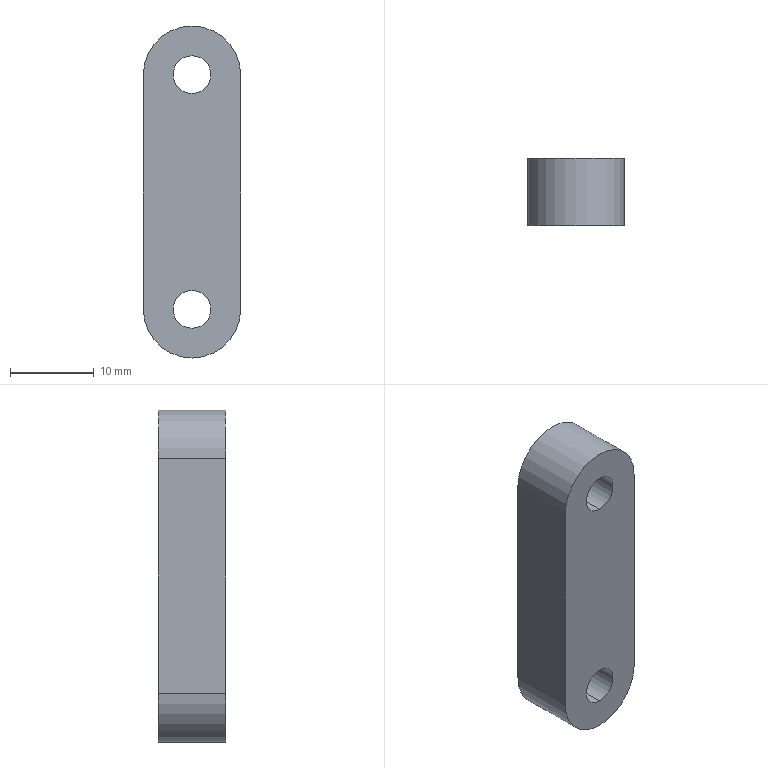Part | SolidWorks | features BaseBody 1 | 1 solid | 17 faces | box 11.6 x 8 x 39.6 mm | volume 2873 mm3 | cylinder 11 | plane 6 | commonest cylinder face diameters 4.5 x4 8 x4 11.6 x3
STEP:
#1=CARTESIAN_POINT('',(-5.8,8.,0.));
#2=VERTEX_POINT('',#1);
#3=CARTESIAN_POINT('',(0.,8.,-5.8));
#4=VERTEX_POINT('',#3);
#5=CARTESIAN_POINT('',(0.,8.,0.));
#6=DIRECTION('',(0.,-1.,0.));
#7=DIRECTION('',(0.,0.,-1.));
#8=AXIS2_PLACEMENT_3D('',#5,#6,#7);
#9=CIRCLE('',#8,5.8);
#10=EDGE_CURVE('',#2,#4,#9,.T.);
#11=ORIENTED_EDGE('',*,*,#10,.T.);
#12=CARTESIAN_POINT('',(0.,0.,-5.8));
#13=VERTEX_POINT('',#12);
#14=CARTESIAN_POINT('',(0.,8.,-5.8));
#15=DIRECTION('',(0.,-1.,0.));
#16=VECTOR('',#15,1000.);
#17=LINE('',#14,#16);
#18=EDGE_CURVE('',#4,#13,#17,.T.);
#19=ORIENTED_EDGE('',*,*,#18,.T.);
#20=CARTESIAN_POINT('',(-5.8,0.,0.));
#21=VERTEX_POINT('',#20);
#22=CARTESIAN_POINT('',(0.,0.,0.));
#23=DIRECTION('',(0.,1.,0.));
#24=DIRECTION('',(0.,0.,-1.));
#25=AXIS2_PLACEMENT_3D('',#22,#23,#24);
#26=CIRCLE('',#25,5.8);
#27=EDGE_CURVE('',#13,#21,#26,.T.);
#28=ORIENTED_EDGE('',*,*,#27,.T.);
#29=CARTESIAN_POINT('',(-5.8,8.,0.));
#30=DIRECTION('',(0.,1.,0.));
#31=VECTOR('',#30,1000.);
#32=LINE('',#29,#31);
#33=EDGE_CURVE('',#21,#2,#32,.T.);
#34=ORIENTED_EDGE('',*,*,#33,.T.);
#35=EDGE_LOOP('',(#11,#19,#28,#34));
#36=FACE_OUTER_BOUND('',#35,.T.);
#37=CARTESIAN_POINT('',(0.,8.,0.));
#38=DIRECTION('',(0.,-1.,0.));
#39=DIRECTION('',(0.,0.,-1.));
#40=AXIS2_PLACEMENT_3D('',#37,#38,#39);
#41=CYLINDRICAL_SURFACE('',#40,5.8);
#42=ADVANCED_FACE('',(#36),#41,.T.);
#43=CARTESIAN_POINT('',(0.,0.,30.25));
#44=VERTEX_POINT('',#43);
#45=CARTESIAN_POINT('',(0.,0.,25.75));
#46=VERTEX_POINT('',#45);
#47=CARTESIAN_POINT('',(0.,0.,28.));
#48=DIRECTION('',(0.,-1.,0.));
#49=DIRECTION('',(0.,0.,1.));
#50=AXIS2_PLACEMENT_3D('',#47,#48,#49);
#51=CIRCLE('',#50,2.25);
#52=EDGE_CURVE('',#44,#46,#51,.T.);
#53=ORIENTED_EDGE('',*,*,#52,.T.);
#54=CARTESIAN_POINT('',(0.,3.4,25.75));
#55=VERTEX_POINT('',#54);
#56=CARTESIAN_POINT('',(0.,8.,25.75));
#57=DIRECTION('',(0.,1.,0.));
#58=VECTOR('',#57,1000.);
#59=LINE('',#56,#58);
#60=EDGE_CURVE('',#46,#55,#59,.T.);
#61=ORIENTED_EDGE('',*,*,#60,.T.);
#62=CARTESIAN_POINT('',(0.,3.4,30.25));
#63=VERTEX_POINT('',#62);
#64=CARTESIAN_POINT('',(0.,3.4,28.));
#65=DIRECTION('',(0.,-1.,0.));
#66=DIRECTION('',(0.,0.,1.));
#67=AXIS2_PLACEMENT_3D('',#64,#65,#66);
#68=CIRCLE('',#67,2.25);
#69=EDGE_CURVE('',#63,#55,#68,.T.);
#70=ORIENTED_EDGE('',*,*,#69,.F.);
#71=CARTESIAN_POINT('',(0.,8.,30.25));
#72=DIRECTION('',(0.,1.,0.));
#73=VECTOR('',#72,1000.);
#74=LINE('',#71,#73);
#75=EDGE_CURVE('',#44,#63,#74,.T.);
#76=ORIENTED_EDGE('',*,*,#75,.F.);
#77=EDGE_LOOP('',(#53,#61,#70,#76));
#78=FACE_OUTER_BOUND('',#77,.T.);
#79=CARTESIAN_POINT('',(0.,8.,28.));
#80=DIRECTION('',(0.,1.,0.));
#81=DIRECTION('',(0.,0.,1.));
#82=AXIS2_PLACEMENT_3D('',#79,#80,#81);
#83=CYLINDRICAL_SURFACE('',#82,2.25);
#84=ADVANCED_FACE('',(#78),#83,.F.);
#85=CARTESIAN_POINT('',(0.,0.,2.25));
#86=VERTEX_POINT('',#85);
#87=CARTESIAN_POINT('',(0.,0.,-2.25));
#88=VERTEX_POINT('',#87);
#89=CARTESIAN_POINT('',(0.,0.,0.));
#90=DIRECTION('',(0.,-1.,0.));
#91=DIRECTION('',(0.,0.,1.));
#92=AXIS2_PLACEMENT_3D('',#89,#90,#91);
#93=CIRCLE('',#92,2.25);
#94=EDGE_CURVE('',#86,#88,#93,.T.);
#95=ORIENTED_EDGE('',*,*,#94,.T.);
#96=CARTESIAN_POINT('',(0.,3.4,-2.25));
#97=VERTEX_POINT('',#96);
#98=CARTESIAN_POINT('',(0.,8.,-2.25));
#99=DIRECTION('',(0.,1.,0.));
#100=VECTOR('',#99,1000.);
#101=LINE('',#98,#100);
#102=EDGE_CURVE('',#88,#97,#101,.T.);
#103=ORIENTED_EDGE('',*,*,#102,.T.);
#104=CARTESIAN_POINT('',(0.,3.4,2.25));
#105=VERTEX_POINT('',#104);
#106=CARTESIAN_POINT('',(0.,3.4,0.));
#107=DIRECTION('',(0.,-1.,0.));
#108=DIRECTION('',(0.,0.,1.));
#109=AXIS2_PLACEMENT_3D('',#106,#107,#108);
#110=CIRCLE('',#109,2.25);
#111=EDGE_CURVE('',#105,#97,#110,.T.);
#112=ORIENTED_EDGE('',*,*,#111,.F.);
#113=CARTESIAN_POINT('',(0.,8.,2.25));
#114=DIRECTION('',(0.,1.,0.));
#115=VECTOR('',#114,1000.);
#116=LINE('',#113,#115);
#117=EDGE_CURVE('',#86,#105,#116,.T.);
#118=ORIENTED_EDGE('',*,*,#117,.F.);
#119=EDGE_LOOP('',(#95,#103,#112,#118));
#120=FACE_OUTER_BOUND('',#119,.T.);
#121=CARTESIAN_POINT('',(0.,8.,0.));
#122=DIRECTION('',(0.,1.,0.));
#123=DIRECTION('',(0.,0.,1.));
#124=AXIS2_PLACEMENT_3D('',#121,#122,#123);
#125=CYLINDRICAL_SURFACE('',#124,2.25);
#126=ADVANCED_FACE('',(#120),#125,.F.);
#127=CARTESIAN_POINT('',(0.,3.4,32.));
#128=VERTEX_POINT('',#127);
#129=CARTESIAN_POINT('',(0.,3.4,24.));
#130=VERTEX_POINT('',#129);
#131=CARTESIAN_POINT('',(0.,3.4,28.));
#132=DIRECTION('',(0.,-1.,0.));
#133=DIRECTION('',(0.,0.,1.));
#134=AXIS2_PLACEMENT_3D('',#131,#132,#133);
#135=CIRCLE('',#134,4.);
#136=EDGE_CURVE('',#128,#130,#135,.T.);
#137=ORIENTED_EDGE('',*,*,#136,.T.);
#138=CARTESIAN_POINT('',(0.,8.,24.));
#139=VERTEX_POINT('',#138);
#140=CARTESIAN_POINT('',(0.,8.,24.));
#141=DIRECTION('',(0.,1.,0.));
#142=VECTOR('',#141,1000.);
#143=LINE('',#140,#142);
#144=EDGE_CURVE('',#130,#139,#143,.T.);
#145=ORIENTED_EDGE('',*,*,#144,.T.);
#146=CARTESIAN_POINT('',(0.,8.,32.));
#147=VERTEX_POINT('',#146);
#148=CARTESIAN_POINT('',(0.,8.,28.));
#149=DIRECTION('',(0.,-1.,0.));
#150=DIRECTION('',(0.,0.,1.));
#151=AXIS2_PLACEMENT_3D('',#148,#149,#150);
#152=CIRCLE('',#151,4.);
#153=EDGE_CURVE('',#147,#139,#152,.T.);
#154=ORIENTED_EDGE('',*,*,#153,.F.);
#155=CARTESIAN_POINT('',(0.,8.,32.));
#156=DIRECTION('',(0.,1.,0.));
#157=VECTOR('',#156,1000.);
#158=LINE('',#155,#157);
#159=EDGE_CURVE('',#128,#147,#158,.T.);
#160=ORIENTED_EDGE('',*,*,#159,.F.);
#161=EDGE_LOOP('',(#137,#145,#154,#160));
#162=FACE_OUTER_BOUND('',#161,.T.);
#163=CARTESIAN_POINT('',(0.,8.,28.));
#164=DIRECTION('',(0.,1.,0.));
#165=DIRECTION('',(0.,0.,1.));
#166=AXIS2_PLACEMENT_3D('',#163,#164,#165);
#167=CYLINDRICAL_SURFACE('',#166,4.);
#168=ADVANCED_FACE('',(#162),#167,.F.);
#169=CARTESIAN_POINT('',(0.,3.4,4.));
#170=VERTEX_POINT('',#169);
#171=CARTESIAN_POINT('',(0.,3.4,-4.));
#172=VERTEX_POINT('',#171);
#173=CARTESIAN_POINT('',(0.,3.4,0.));
#174=DIRECTION('',(0.,-1.,0.));
#175=DIRECTION('',(0.,0.,1.));
#176=AXIS2_PLACEMENT_3D('',#173,#174,#175);
#177=CIRCLE('',#176,4.);
#178=EDGE_CURVE('',#170,#172,#177,.T.);
#179=ORIENTED_EDGE('',*,*,#178,.T.);
#180=CARTESIAN_POINT('',(0.,8.,-4.));
#181=VERTEX_POINT('',#180);
#182=CARTESIAN_POINT('',(0.,8.,-4.));
#183=DIRECTION('',(0.,1.,0.));
#184=VECTOR('',#183,1000.);
#185=LINE('',#182,#184);
#186=EDGE_CURVE('',#172,#181,#185,.T.);
#187=ORIENTED_EDGE('',*,*,#186,.T.);
#188=CARTESIAN_POINT('',(0.,8.,4.));
#189=VERTEX_POINT('',#188);
#190=CARTESIAN_POINT('',(0.,8.,0.));
#191=DIRECTION('',(0.,-1.,0.));
#192=DIRECTION('',(0.,0.,1.));
#193=AXIS2_PLACEMENT_3D('',#190,#191,#192);
#194=CIRCLE('',#193,4.);
#195=EDGE_CURVE('',#189,#181,#194,.T.);
#196=ORIENTED_EDGE('',*,*,#195,.F.);
#197=CARTESIAN_POINT('',(0.,8.,4.));
#198=DIRECTION('',(0.,1.,0.));
#199=VECTOR('',#198,1000.);
#200=LINE('',#197,#199);
#201=EDGE_CURVE('',#170,#189,#200,.T.);
#202=ORIENTED_EDGE('',*,*,#201,.F.);
#203=EDGE_LOOP('',(#179,#187,#196,#202));
#204=FACE_OUTER_BOUND('',#203,.T.);
#205=CARTESIAN_POINT('',(0.,8.,0.));
#206=DIRECTION('',(0.,1.,0.));
#207=DIRECTION('',(0.,0.,1.));
#208=AXIS2_PLACEMENT_3D('',#205,#206,#207);
#209=CYLINDRICAL_SURFACE('',#208,4.);
#210=ADVANCED_FACE('',(#204),#209,.F.);
#211=CARTESIAN_POINT('',(5.8,0.,28.));
#212=VERTEX_POINT('',#211);
#213=CARTESIAN_POINT('',(5.8,0.,0.));
#214=VERTEX_POINT('',#213);
#215=CARTESIAN_POINT('',(5.8,0.,0.));
#216=DIRECTION('',(0.,0.,-1.));
#217=VECTOR('',#216,1000.);
#218=LINE('',#215,#217);
#219=EDGE_CURVE('',#212,#214,#218,.T.);
#220=ORIENTED_EDGE('',*,*,#219,.F.);
#221=CARTESIAN_POINT('',(-5.8,0.,28.));
#222=VERTEX_POINT('',#221);
#223=CARTESIAN_POINT('',(0.,0.,28.));
#224=DIRECTION('',(0.,1.,0.));
#225=DIRECTION('',(0.,0.,-1.));
#226=AXIS2_PLACEMENT_3D('',#223,#224,#225);
#227=CIRCLE('',#226,5.8);
#228=EDGE_CURVE('',#222,#212,#227,.T.);
#229=ORIENTED_EDGE('',*,*,#228,.F.);
#230=CARTESIAN_POINT('',(-5.8,0.,0.));
#231=DIRECTION('',(0.,0.,1.));
#232=VECTOR('',#231,1000.);
#233=LINE('',#230,#232);
#234=EDGE_CURVE('',#21,#222,#233,.T.);
#235=ORIENTED_EDGE('',*,*,#234,.F.);
#236=ORIENTED_EDGE('',*,*,#27,.F.);
#237=CARTESIAN_POINT('',(0.,0.,0.));
#238=DIRECTION('',(0.,1.,0.));
#239=DIRECTION('',(0.,0.,-1.));
#240=AXIS2_PLACEMENT_3D('',#237,#238,#239);
#241=CIRCLE('',#240,5.8);
#242=EDGE_CURVE('',#214,#13,#241,.T.);
#243=ORIENTED_EDGE('',*,*,#242,.F.);
#244=EDGE_LOOP('',(#220,#229,#235,#236,#243));
#245=FACE_OUTER_BOUND('',#244,.T.);
#246=ORIENTED_EDGE('',*,*,#52,.F.);
#247=CARTESIAN_POINT('',(0.,0.,28.));
#248=DIRECTION('',(0.,-1.,0.));
#249=DIRECTION('',(0.,0.,1.));
#250=AXIS2_PLACEMENT_3D('',#247,#248,#249);
#251=CIRCLE('',#250,2.25);
#252=EDGE_CURVE('',#46,#44,#251,.T.);
#253=ORIENTED_EDGE('',*,*,#252,.F.);
#254=EDGE_LOOP('',(#246,#253));
#255=FACE_BOUND('',#254,.T.);
#256=ORIENTED_EDGE('',*,*,#94,.F.);
#257=CARTESIAN_POINT('',(0.,0.,0.));
#258=DIRECTION('',(0.,-1.,0.));
#259=DIRECTION('',(0.,0.,1.));
#260=AXIS2_PLACEMENT_3D('',#257,#258,#259);
#261=CIRCLE('',#260,2.25);
#262=EDGE_CURVE('',#88,#86,#261,.T.);
#263=ORIENTED_EDGE('',*,*,#262,.F.);
#264=EDGE_LOOP('',(#256,#263));
#265=FACE_BOUND('',#264,.T.);
#266=CARTESIAN_POINT('',(0.,0.,0.));
#267=DIRECTION('',(0.,1.,0.));
#268=DIRECTION('',(0.,0.,1.));
#269=AXIS2_PLACEMENT_3D('',#266,#267,#268);
#270=PLANE('',#269);
#271=ADVANCED_FACE('',(#245,#255,#265),#270,.F.);
#272=ORIENTED_EDGE('',*,*,#18,.F.);
#273=CARTESIAN_POINT('',(5.8,8.,0.));
#274=VERTEX_POINT('',#273);
#275=CARTESIAN_POINT('',(0.,8.,0.));
#276=DIRECTION('',(0.,-1.,0.));
#277=DIRECTION('',(0.,0.,-1.));
#278=AXIS2_PLACEMENT_3D('',#275,#276,#277);
#279=CIRCLE('',#278,5.8);
#280=EDGE_CURVE('',#4,#274,#279,.T.);
#281=ORIENTED_EDGE('',*,*,#280,.T.);
#282=CARTESIAN_POINT('',(5.8,8.,0.));
#283=DIRECTION('',(0.,-1.,0.));
#284=VECTOR('',#283,1000.);
#285=LINE('',#282,#284);
#286=EDGE_CURVE('',#274,#214,#285,.T.);
#287=ORIENTED_EDGE('',*,*,#286,.T.);
#288=ORIENTED_EDGE('',*,*,#242,.T.);
#289=EDGE_LOOP('',(#272,#281,#287,#288));
#290=FACE_OUTER_BOUND('',#289,.T.);
#291=CARTESIAN_POINT('',(0.,8.,0.));
#292=DIRECTION('',(0.,-1.,0.));
#293=DIRECTION('',(0.,0.,-1.));
#294=AXIS2_PLACEMENT_3D('',#291,#292,#293);
#295=CYLINDRICAL_SURFACE('',#294,5.8);
#296=ADVANCED_FACE('',(#290),#295,.T.);
#297=ORIENTED_EDGE('',*,*,#286,.F.);
#298=CARTESIAN_POINT('',(5.8,8.,28.));
#299=VERTEX_POINT('',#298);
#300=CARTESIAN_POINT('',(5.8,8.,0.));
#301=DIRECTION('',(0.,0.,-1.));
#302=VECTOR('',#301,1000.);
#303=LINE('',#300,#302);
#304=EDGE_CURVE('',#299,#274,#303,.T.);
#305=ORIENTED_EDGE('',*,*,#304,.F.);
#306=CARTESIAN_POINT('',(5.8,8.,28.));
#307=DIRECTION('',(0.,1.,0.));
#308=VECTOR('',#307,1000.);
#309=LINE('',#306,#308);
#310=EDGE_CURVE('',#212,#299,#309,.T.);
#311=ORIENTED_EDGE('',*,*,#310,.F.);
#312=ORIENTED_EDGE('',*,*,#219,.T.);
#313=EDGE_LOOP('',(#297,#305,#311,#312));
#314=FACE_OUTER_BOUND('',#313,.T.);
#315=CARTESIAN_POINT('',(5.8,8.,0.));
#316=DIRECTION('',(-1.,0.,0.));
#317=DIRECTION('',(0.,0.,1.));
#318=AXIS2_PLACEMENT_3D('',#315,#316,#317);
#319=PLANE('',#318);
#320=ADVANCED_FACE('',(#314),#319,.F.);
#321=CARTESIAN_POINT('',(-5.8,8.,28.));
#322=VERTEX_POINT('',#321);
#323=CARTESIAN_POINT('',(0.,8.,28.));
#324=DIRECTION('',(0.,-1.,0.));
#325=DIRECTION('',(0.,0.,-1.));
#326=AXIS2_PLACEMENT_3D('',#323,#324,#325);
#327=CIRCLE('',#326,5.8);
#328=EDGE_CURVE('',#299,#322,#327,.T.);
#329=ORIENTED_EDGE('',*,*,#328,.T.);
#330=CARTESIAN_POINT('',(-5.8,8.,28.));
#331=DIRECTION('',(0.,-1.,0.));
#332=VECTOR('',#331,1000.);
#333=LINE('',#330,#332);
#334=EDGE_CURVE('',#322,#222,#333,.T.);
#335=ORIENTED_EDGE('',*,*,#334,.T.);
#336=ORIENTED_EDGE('',*,*,#228,.T.);
#337=ORIENTED_EDGE('',*,*,#310,.T.);
#338=EDGE_LOOP('',(#329,#335,#336,#337));
#339=FACE_OUTER_BOUND('',#338,.T.);
#340=CARTESIAN_POINT('',(0.,8.,28.));
#341=DIRECTION('',(0.,-1.,0.));
#342=DIRECTION('',(0.,0.,-1.));
#343=AXIS2_PLACEMENT_3D('',#340,#341,#342);
#344=CYLINDRICAL_SURFACE('',#343,5.8);
#345=ADVANCED_FACE('',(#339),#344,.T.);
#346=ORIENTED_EDGE('',*,*,#334,.F.);
#347=CARTESIAN_POINT('',(-5.8,8.,0.));
#348=DIRECTION('',(0.,0.,1.));
#349=VECTOR('',#348,1000.);
#350=LINE('',#347,#349);
#351=EDGE_CURVE('',#2,#322,#350,.T.);
#352=ORIENTED_EDGE('',*,*,#351,.F.);
#353=ORIENTED_EDGE('',*,*,#33,.F.);
#354=ORIENTED_EDGE('',*,*,#234,.T.);
#355=EDGE_LOOP('',(#346,#352,#353,#354));
#356=FACE_OUTER_BOUND('',#355,.T.);
#357=CARTESIAN_POINT('',(-5.8,8.,0.));
#358=DIRECTION('',(1.,0.,0.));
#359=DIRECTION('',(0.,0.,-1.));
#360=AXIS2_PLACEMENT_3D('',#357,#358,#359);
#361=PLANE('',#360);
#362=ADVANCED_FACE('',(#356),#361,.F.);
#363=ORIENTED_EDGE('',*,*,#60,.F.);
#364=ORIENTED_EDGE('',*,*,#252,.T.);
#365=ORIENTED_EDGE('',*,*,#75,.T.);
#366=CARTESIAN_POINT('',(0.,3.4,28.));
#367=DIRECTION('',(0.,-1.,0.));
#368=DIRECTION('',(0.,0.,1.));
#369=AXIS2_PLACEMENT_3D('',#366,#367,#368);
#370=CIRCLE('',#369,2.25);
#371=EDGE_CURVE('',#55,#63,#370,.T.);
#372=ORIENTED_EDGE('',*,*,#371,.F.);
#373=EDGE_LOOP('',(#363,#364,#365,#372));
#374=FACE_OUTER_BOUND('',#373,.T.);
#375=CARTESIAN_POINT('',(0.,8.,28.));
#376=DIRECTION('',(0.,1.,0.));
#377=DIRECTION('',(0.,0.,1.));
#378=AXIS2_PLACEMENT_3D('',#375,#376,#377);
#379=CYLINDRICAL_SURFACE('',#378,2.25);
#380=ADVANCED_FACE('',(#374),#379,.F.);
#381=ORIENTED_EDGE('',*,*,#102,.F.);
#382=ORIENTED_EDGE('',*,*,#262,.T.);
#383=ORIENTED_EDGE('',*,*,#117,.T.);
#384=CARTESIAN_POINT('',(0.,3.4,0.));
#385=DIRECTION('',(0.,-1.,0.));
#386=DIRECTION('',(0.,0.,1.));
#387=AXIS2_PLACEMENT_3D('',#384,#385,#386);
#388=CIRCLE('',#387,2.25);
#389=EDGE_CURVE('',#97,#105,#388,.T.);
#390=ORIENTED_EDGE('',*,*,#389,.F.);
#391=EDGE_LOOP('',(#381,#382,#383,#390));
#392=FACE_OUTER_BOUND('',#391,.T.);
#393=CARTESIAN_POINT('',(0.,8.,0.));
#394=DIRECTION('',(0.,1.,0.));
#395=DIRECTION('',(0.,0.,1.));
#396=AXIS2_PLACEMENT_3D('',#393,#394,#395);
#397=CYLINDRICAL_SURFACE('',#396,2.25);
#398=ADVANCED_FACE('',(#392),#397,.F.);
#399=ORIENTED_EDGE('',*,*,#328,.F.);
#400=ORIENTED_EDGE('',*,*,#304,.T.);
#401=ORIENTED_EDGE('',*,*,#280,.F.);
#402=ORIENTED_EDGE('',*,*,#10,.F.);
#403=ORIENTED_EDGE('',*,*,#351,.T.);
#404=EDGE_LOOP('',(#399,#400,#401,#402,#403));
#405=FACE_OUTER_BOUND('',#404,.T.);
#406=ORIENTED_EDGE('',*,*,#153,.T.);
#407=CARTESIAN_POINT('',(0.,8.,28.));
#408=DIRECTION('',(0.,-1.,0.));
#409=DIRECTION('',(0.,0.,1.));
#410=AXIS2_PLACEMENT_3D('',#407,#408,#409);
#411=CIRCLE('',#410,4.);
#412=EDGE_CURVE('',#139,#147,#411,.T.);
#413=ORIENTED_EDGE('',*,*,#412,.T.);
#414=EDGE_LOOP('',(#406,#413));
#415=FACE_BOUND('',#414,.T.);
#416=ORIENTED_EDGE('',*,*,#195,.T.);
#417=CARTESIAN_POINT('',(0.,8.,0.));
#418=DIRECTION('',(0.,-1.,0.));
#419=DIRECTION('',(0.,0.,1.));
#420=AXIS2_PLACEMENT_3D('',#417,#418,#419);
#421=CIRCLE('',#420,4.);
#422=EDGE_CURVE('',#181,#189,#421,.T.);
#423=ORIENTED_EDGE('',*,*,#422,.T.);
#424=EDGE_LOOP('',(#416,#423));
#425=FACE_BOUND('',#424,.T.);
#426=CARTESIAN_POINT('',(0.,8.,0.));
#427=DIRECTION('',(0.,1.,0.));
#428=DIRECTION('',(0.,0.,1.));
#429=AXIS2_PLACEMENT_3D('',#426,#427,#428);
#430=PLANE('',#429);
#431=ADVANCED_FACE('',(#405,#415,#425),#430,.T.);
#432=ORIENTED_EDGE('',*,*,#136,.F.);
#433=CARTESIAN_POINT('',(0.,3.4,28.));
#434=DIRECTION('',(0.,-1.,0.));
#435=DIRECTION('',(0.,0.,1.));
#436=AXIS2_PLACEMENT_3D('',#433,#434,#435);
#437=CIRCLE('',#436,4.);
#438=EDGE_CURVE('',#130,#128,#437,.T.);
#439=ORIENTED_EDGE('',*,*,#438,.F.);
#440=EDGE_LOOP('',(#432,#439));
#441=FACE_OUTER_BOUND('',#440,.T.);
#442=ORIENTED_EDGE('',*,*,#69,.T.);
#443=ORIENTED_EDGE('',*,*,#371,.T.);
#444=EDGE_LOOP('',(#442,#443));
#445=FACE_BOUND('',#444,.T.);
#446=CARTESIAN_POINT('',(2.25,3.4,28.));
#447=DIRECTION('',(0.,-1.,0.));
#448=DIRECTION('',(0.,0.,-1.));
#449=AXIS2_PLACEMENT_3D('',#446,#447,#448);
#450=PLANE('',#449);
#451=ADVANCED_FACE('',(#441,#445),#450,.F.);
#452=ORIENTED_EDGE('',*,*,#178,.F.);
#453=CARTESIAN_POINT('',(0.,3.4,0.));
#454=DIRECTION('',(0.,-1.,0.));
#455=DIRECTION('',(0.,0.,1.));
#456=AXIS2_PLACEMENT_3D('',#453,#454,#455);
#457=CIRCLE('',#456,4.);
#458=EDGE_CURVE('',#172,#170,#457,.T.);
#459=ORIENTED_EDGE('',*,*,#458,.F.);
#460=EDGE_LOOP('',(#452,#459));
#461=FACE_OUTER_BOUND('',#460,.T.);
#462=ORIENTED_EDGE('',*,*,#111,.T.);
#463=ORIENTED_EDGE('',*,*,#389,.T.);
#464=EDGE_LOOP('',(#462,#463));
#465=FACE_BOUND('',#464,.T.);
#466=CARTESIAN_POINT('',(2.25,3.4,0.));
#467=DIRECTION('',(0.,-1.,0.));
#468=DIRECTION('',(0.,0.,-1.));
#469=AXIS2_PLACEMENT_3D('',#466,#467,#468);
#470=PLANE('',#469);
#471=ADVANCED_FACE('',(#461,#465),#470,.F.);
#472=ORIENTED_EDGE('',*,*,#144,.F.);
#473=ORIENTED_EDGE('',*,*,#438,.T.);
#474=ORIENTED_EDGE('',*,*,#159,.T.);
#475=ORIENTED_EDGE('',*,*,#412,.F.);
#476=EDGE_LOOP('',(#472,#473,#474,#475));
#477=FACE_OUTER_BOUND('',#476,.T.);
#478=CARTESIAN_POINT('',(0.,8.,28.));
#479=DIRECTION('',(0.,1.,0.));
#480=DIRECTION('',(0.,0.,1.));
#481=AXIS2_PLACEMENT_3D('',#478,#479,#480);
#482=CYLINDRICAL_SURFACE('',#481,4.);
#483=ADVANCED_FACE('',(#477),#482,.F.);
#484=ORIENTED_EDGE('',*,*,#186,.F.);
#485=ORIENTED_EDGE('',*,*,#458,.T.);
#486=ORIENTED_EDGE('',*,*,#201,.T.);
#487=ORIENTED_EDGE('',*,*,#422,.F.);
#488=EDGE_LOOP('',(#484,#485,#486,#487));
#489=FACE_OUTER_BOUND('',#488,.T.);
#490=CARTESIAN_POINT('',(0.,8.,0.));
#491=DIRECTION('',(0.,1.,0.));
#492=DIRECTION('',(0.,0.,1.));
#493=AXIS2_PLACEMENT_3D('',#490,#491,#492);
#494=CYLINDRICAL_SURFACE('',#493,4.);
#495=ADVANCED_FACE('',(#489),#494,.F.);
#496=CLOSED_SHELL('',(#42,#84,#126,#168,#210,#271,#296,#320,#345,#362,#380,#398,#431,#451,#471,#483,#495));
#497=MANIFOLD_SOLID_BREP('',#496);
#498=CARTESIAN_POINT('',(0.,0.,0.));
#499=DIRECTION('',(0.,0.,1.));
#500=DIRECTION('',(1.,0.,0.));
#501=AXIS2_PLACEMENT_3D('',#498,#499,#500);
#502=(LENGTH_UNIT()NAMED_UNIT(*)SI_UNIT(.MILLI.,.METRE.));
#503=UNCERTAINTY_MEASURE_WITH_UNIT(LENGTH_MEASURE(0.00001),#502,'','');
#504=(NAMED_UNIT(*)PLANE_ANGLE_UNIT()SI_UNIT($,.RADIAN.));
#505=(NAMED_UNIT(*)SI_UNIT($,.STERADIAN.)SOLID_ANGLE_UNIT());
#506=(GEOMETRIC_REPRESENTATION_CONTEXT(3)GLOBAL_UNCERTAINTY_ASSIGNED_CONTEXT((#503))GLOBAL_UNIT_ASSIGNED_CONTEXT((#502,#504,#505))REPRESENTATION_CONTEXT('',''));
#507=ADVANCED_BREP_SHAPE_REPRESENTATION('',(#497,#501),#506);